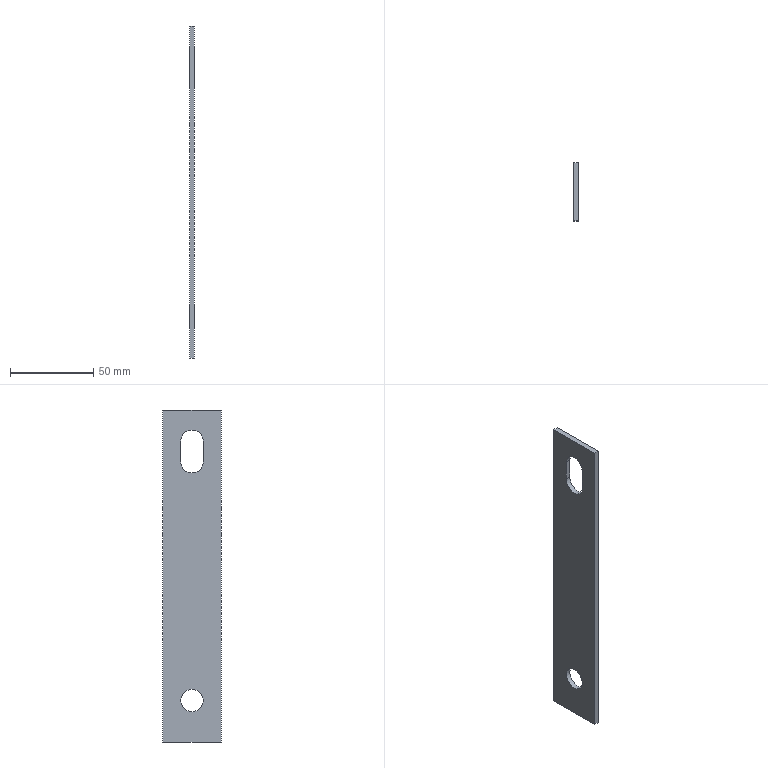Part | NX | features solid 2 | 1 solid | 11 faces | box 3 x 35 x 200 mm | volume 19635 mm3 | plane 8 | cylinder 3 | commonest cylinder face diameters 13.5 x3
STEP:
#1=CARTESIAN_POINT('',(1620.,-182.5,-320.));
#2=VERTEX_POINT('',#1);
#3=CARTESIAN_POINT('',(1620.,-182.5,-120.));
#4=VERTEX_POINT('',#3);
#5=CARTESIAN_POINT('',(1620.,-182.5,-320.));
#6=DIRECTION('',(0.,0.,1.));
#7=VECTOR('',#6,1000.);
#8=LINE('',#5,#7);
#9=EDGE_CURVE('',#2,#4,#8,.T.);
#10=ORIENTED_EDGE('',*,*,#9,.F.);
#11=CARTESIAN_POINT('',(1623.,-182.5,-320.));
#12=VERTEX_POINT('',#11);
#13=CARTESIAN_POINT('',(1623.,-182.5,-320.));
#14=DIRECTION('',(-1.,0.,0.));
#15=VECTOR('',#14,1000.);
#16=LINE('',#13,#15);
#17=EDGE_CURVE('',#12,#2,#16,.T.);
#18=ORIENTED_EDGE('',*,*,#17,.F.);
#19=CARTESIAN_POINT('',(1623.,-182.5,-120.));
#20=VERTEX_POINT('',#19);
#21=CARTESIAN_POINT('',(1623.,-182.5,-320.));
#22=DIRECTION('',(0.,0.,1.));
#23=VECTOR('',#22,1000.);
#24=LINE('',#21,#23);
#25=EDGE_CURVE('',#12,#20,#24,.T.);
#26=ORIENTED_EDGE('',*,*,#25,.T.);
#27=CARTESIAN_POINT('',(1623.,-182.5,-120.));
#28=DIRECTION('',(-1.,0.,0.));
#29=VECTOR('',#28,1000.);
#30=LINE('',#27,#29);
#31=EDGE_CURVE('',#20,#4,#30,.T.);
#32=ORIENTED_EDGE('',*,*,#31,.T.);
#33=EDGE_LOOP('',(#10,#18,#26,#32));
#34=FACE_BOUND('',#33,.T.);
#35=CARTESIAN_POINT('',(1623.,-182.5,-320.));
#36=DIRECTION('',(0.,-1.,0.));
#37=DIRECTION('',(0.,0.,1.));
#38=AXIS2_PLACEMENT_3D('',#35,#36,#37);
#39=PLANE('',#38);
#40=ADVANCED_FACE('',(#34),#39,.T.);
#41=CARTESIAN_POINT('',(1620.,-147.5,-120.));
#42=VERTEX_POINT('',#41);
#43=CARTESIAN_POINT('',(1620.,-182.5,-120.));
#44=DIRECTION('',(0.,1.,0.));
#45=VECTOR('',#44,1000.);
#46=LINE('',#43,#45);
#47=EDGE_CURVE('',#4,#42,#46,.T.);
#48=ORIENTED_EDGE('',*,*,#47,.F.);
#49=ORIENTED_EDGE('',*,*,#31,.F.);
#50=CARTESIAN_POINT('',(1623.,-147.5,-120.));
#51=VERTEX_POINT('',#50);
#52=CARTESIAN_POINT('',(1623.,-182.5,-120.));
#53=DIRECTION('',(0.,1.,0.));
#54=VECTOR('',#53,1000.);
#55=LINE('',#52,#54);
#56=EDGE_CURVE('',#20,#51,#55,.T.);
#57=ORIENTED_EDGE('',*,*,#56,.T.);
#58=CARTESIAN_POINT('',(1623.,-147.5,-120.));
#59=DIRECTION('',(-1.,0.,0.));
#60=VECTOR('',#59,1000.);
#61=LINE('',#58,#60);
#62=EDGE_CURVE('',#51,#42,#61,.T.);
#63=ORIENTED_EDGE('',*,*,#62,.T.);
#64=EDGE_LOOP('',(#48,#49,#57,#63));
#65=FACE_BOUND('',#64,.T.);
#66=CARTESIAN_POINT('',(1623.,-182.5,-120.));
#67=DIRECTION('',(0.,0.,1.));
#68=DIRECTION('',(-1.,0.,0.));
#69=AXIS2_PLACEMENT_3D('',#66,#67,#68);
#70=PLANE('',#69);
#71=ADVANCED_FACE('',(#65),#70,.T.);
#72=CARTESIAN_POINT('',(1620.,-147.5,-320.));
#73=VERTEX_POINT('',#72);
#74=CARTESIAN_POINT('',(1620.,-147.5,-120.));
#75=DIRECTION('',(0.,0.,-1.));
#76=VECTOR('',#75,1000.);
#77=LINE('',#74,#76);
#78=EDGE_CURVE('',#42,#73,#77,.T.);
#79=ORIENTED_EDGE('',*,*,#78,.F.);
#80=ORIENTED_EDGE('',*,*,#62,.F.);
#81=CARTESIAN_POINT('',(1623.,-147.5,-320.));
#82=VERTEX_POINT('',#81);
#83=CARTESIAN_POINT('',(1623.,-147.5,-120.));
#84=DIRECTION('',(0.,0.,-1.));
#85=VECTOR('',#84,1000.);
#86=LINE('',#83,#85);
#87=EDGE_CURVE('',#51,#82,#86,.T.);
#88=ORIENTED_EDGE('',*,*,#87,.T.);
#89=CARTESIAN_POINT('',(1623.,-147.5,-320.));
#90=DIRECTION('',(-1.,0.,0.));
#91=VECTOR('',#90,1000.);
#92=LINE('',#89,#91);
#93=EDGE_CURVE('',#82,#73,#92,.T.);
#94=ORIENTED_EDGE('',*,*,#93,.T.);
#95=EDGE_LOOP('',(#79,#80,#88,#94));
#96=FACE_BOUND('',#95,.T.);
#97=CARTESIAN_POINT('',(1623.,-147.5,-120.));
#98=DIRECTION('',(0.,1.,0.));
#99=DIRECTION('',(0.,0.,-1.));
#100=AXIS2_PLACEMENT_3D('',#97,#98,#99);
#101=PLANE('',#100);
#102=ADVANCED_FACE('',(#96),#101,.T.);
#103=CARTESIAN_POINT('',(1620.,-158.25,-151.25));
#104=VERTEX_POINT('',#103);
#105=CARTESIAN_POINT('',(1620.,-171.75,-151.25));
#106=VERTEX_POINT('',#105);
#107=CARTESIAN_POINT('',(1620.,-165.,-151.25));
#108=DIRECTION('',(-1.,0.,0.));
#109=DIRECTION('',(0.,-1.,0.));
#110=AXIS2_PLACEMENT_3D('',#107,#108,#109);
#111=CIRCLE('',#110,6.75);
#112=EDGE_CURVE('',#104,#106,#111,.T.);
#113=ORIENTED_EDGE('',*,*,#112,.T.);
#114=CARTESIAN_POINT('',(1623.,-171.75,-151.25));
#115=VERTEX_POINT('',#114);
#116=CARTESIAN_POINT('',(1623.,-171.75,-151.25));
#117=DIRECTION('',(-1.,0.,0.));
#118=VECTOR('',#117,1000.);
#119=LINE('',#116,#118);
#120=EDGE_CURVE('',#115,#106,#119,.T.);
#121=ORIENTED_EDGE('',*,*,#120,.F.);
#122=CARTESIAN_POINT('',(1623.,-158.25,-151.25));
#123=VERTEX_POINT('',#122);
#124=CARTESIAN_POINT('',(1623.,-165.,-151.25));
#125=DIRECTION('',(-1.,0.,0.));
#126=DIRECTION('',(0.,-1.,0.));
#127=AXIS2_PLACEMENT_3D('',#124,#125,#126);
#128=CIRCLE('',#127,6.75);
#129=EDGE_CURVE('',#123,#115,#128,.T.);
#130=ORIENTED_EDGE('',*,*,#129,.F.);
#131=CARTESIAN_POINT('',(1623.,-158.25,-151.25));
#132=DIRECTION('',(-1.,0.,0.));
#133=VECTOR('',#132,1000.);
#134=LINE('',#131,#133);
#135=EDGE_CURVE('',#123,#104,#134,.T.);
#136=ORIENTED_EDGE('',*,*,#135,.T.);
#137=EDGE_LOOP('',(#113,#121,#130,#136));
#138=FACE_BOUND('',#137,.T.);
#139=CARTESIAN_POINT('',(1623.,-165.,-151.25));
#140=DIRECTION('',(-1.,0.,0.));
#141=DIRECTION('',(0.,-1.,0.));
#142=AXIS2_PLACEMENT_3D('',#139,#140,#141);
#143=CYLINDRICAL_SURFACE('',#142,6.75);
#144=ADVANCED_FACE('',(#138),#143,.F.);
#145=CARTESIAN_POINT('',(1620.,-158.25,-138.75));
#146=VERTEX_POINT('',#145);
#147=CARTESIAN_POINT('',(1620.,-158.25,-151.25));
#148=DIRECTION('',(0.,0.,1.));
#149=VECTOR('',#148,1000.);
#150=LINE('',#147,#149);
#151=EDGE_CURVE('',#104,#146,#150,.T.);
#152=ORIENTED_EDGE('',*,*,#151,.F.);
#153=ORIENTED_EDGE('',*,*,#135,.F.);
#154=CARTESIAN_POINT('',(1623.,-158.25,-138.75));
#155=VERTEX_POINT('',#154);
#156=CARTESIAN_POINT('',(1623.,-158.25,-151.25));
#157=DIRECTION('',(0.,0.,1.));
#158=VECTOR('',#157,1000.);
#159=LINE('',#156,#158);
#160=EDGE_CURVE('',#123,#155,#159,.T.);
#161=ORIENTED_EDGE('',*,*,#160,.T.);
#162=CARTESIAN_POINT('',(1623.,-158.25,-138.75));
#163=DIRECTION('',(-1.,0.,0.));
#164=VECTOR('',#163,1000.);
#165=LINE('',#162,#164);
#166=EDGE_CURVE('',#155,#146,#165,.T.);
#167=ORIENTED_EDGE('',*,*,#166,.T.);
#168=EDGE_LOOP('',(#152,#153,#161,#167));
#169=FACE_BOUND('',#168,.T.);
#170=CARTESIAN_POINT('',(1623.,-158.25,-151.25));
#171=DIRECTION('',(0.,-1.,0.));
#172=DIRECTION('',(1.,0.,0.));
#173=AXIS2_PLACEMENT_3D('',#170,#171,#172);
#174=PLANE('',#173);
#175=ADVANCED_FACE('',(#169),#174,.T.);
#176=CARTESIAN_POINT('',(1620.,-171.75,-138.75));
#177=VERTEX_POINT('',#176);
#178=CARTESIAN_POINT('',(1620.,-165.,-138.75));
#179=DIRECTION('',(-1.,0.,0.));
#180=DIRECTION('',(0.,-1.,0.));
#181=AXIS2_PLACEMENT_3D('',#178,#179,#180);
#182=CIRCLE('',#181,6.75);
#183=EDGE_CURVE('',#177,#146,#182,.T.);
#184=ORIENTED_EDGE('',*,*,#183,.T.);
#185=ORIENTED_EDGE('',*,*,#166,.F.);
#186=CARTESIAN_POINT('',(1623.,-171.75,-138.75));
#187=VERTEX_POINT('',#186);
#188=CARTESIAN_POINT('',(1623.,-165.,-138.75));
#189=DIRECTION('',(-1.,0.,0.));
#190=DIRECTION('',(0.,-1.,0.));
#191=AXIS2_PLACEMENT_3D('',#188,#189,#190);
#192=CIRCLE('',#191,6.75);
#193=EDGE_CURVE('',#187,#155,#192,.T.);
#194=ORIENTED_EDGE('',*,*,#193,.F.);
#195=CARTESIAN_POINT('',(1623.,-171.75,-138.75));
#196=DIRECTION('',(-1.,0.,0.));
#197=VECTOR('',#196,1000.);
#198=LINE('',#195,#197);
#199=EDGE_CURVE('',#187,#177,#198,.T.);
#200=ORIENTED_EDGE('',*,*,#199,.T.);
#201=EDGE_LOOP('',(#184,#185,#194,#200));
#202=FACE_BOUND('',#201,.T.);
#203=CARTESIAN_POINT('',(1623.,-165.,-138.75));
#204=DIRECTION('',(-1.,0.,0.));
#205=DIRECTION('',(0.,-1.,0.));
#206=AXIS2_PLACEMENT_3D('',#203,#204,#205);
#207=CYLINDRICAL_SURFACE('',#206,6.75);
#208=ADVANCED_FACE('',(#202),#207,.F.);
#209=CARTESIAN_POINT('',(1620.,-171.75,-138.75));
#210=DIRECTION('',(0.,0.,-1.));
#211=VECTOR('',#210,1000.);
#212=LINE('',#209,#211);
#213=EDGE_CURVE('',#177,#106,#212,.T.);
#214=ORIENTED_EDGE('',*,*,#213,.F.);
#215=ORIENTED_EDGE('',*,*,#199,.F.);
#216=CARTESIAN_POINT('',(1623.,-171.75,-138.75));
#217=DIRECTION('',(0.,0.,-1.));
#218=VECTOR('',#217,1000.);
#219=LINE('',#216,#218);
#220=EDGE_CURVE('',#187,#115,#219,.T.);
#221=ORIENTED_EDGE('',*,*,#220,.T.);
#222=ORIENTED_EDGE('',*,*,#120,.T.);
#223=EDGE_LOOP('',(#214,#215,#221,#222));
#224=FACE_BOUND('',#223,.T.);
#225=CARTESIAN_POINT('',(1623.,-171.75,-138.75));
#226=DIRECTION('',(0.,1.,0.));
#227=DIRECTION('',(-1.,0.,0.));
#228=AXIS2_PLACEMENT_3D('',#225,#226,#227);
#229=PLANE('',#228);
#230=ADVANCED_FACE('',(#224),#229,.T.);
#231=CARTESIAN_POINT('',(1623.,-171.75,-295.));
#232=VERTEX_POINT('',#231);
#233=CARTESIAN_POINT('',(1623.,-165.,-295.));
#234=DIRECTION('',(-1.,0.,0.));
#235=DIRECTION('',(0.,-1.,0.));
#236=AXIS2_PLACEMENT_3D('',#233,#234,#235);
#237=CIRCLE('',#236,6.75);
#238=EDGE_CURVE('',#232,#232,#237,.T.);
#239=ORIENTED_EDGE('',*,*,#238,.F.);
#240=EDGE_LOOP('',(#239));
#241=FACE_BOUND('',#240,.T.);
#242=CARTESIAN_POINT('',(1620.,-171.75,-295.));
#243=VERTEX_POINT('',#242);
#244=CARTESIAN_POINT('',(1620.,-165.,-295.));
#245=DIRECTION('',(-1.,0.,0.));
#246=DIRECTION('',(0.,-1.,0.));
#247=AXIS2_PLACEMENT_3D('',#244,#245,#246);
#248=CIRCLE('',#247,6.75);
#249=EDGE_CURVE('',#243,#243,#248,.T.);
#250=ORIENTED_EDGE('',*,*,#249,.T.);
#251=EDGE_LOOP('',(#250));
#252=FACE_BOUND('',#251,.T.);
#253=CARTESIAN_POINT('',(1623.,-165.,-295.));
#254=DIRECTION('',(-1.,0.,0.));
#255=DIRECTION('',(0.,-1.,0.));
#256=AXIS2_PLACEMENT_3D('',#253,#254,#255);
#257=CYLINDRICAL_SURFACE('',#256,6.75);
#258=ADVANCED_FACE('',(#241,#252),#257,.F.);
#259=CARTESIAN_POINT('',(1620.,-147.5,-320.));
#260=DIRECTION('',(0.,-1.,0.));
#261=VECTOR('',#260,1000.);
#262=LINE('',#259,#261);
#263=EDGE_CURVE('',#73,#2,#262,.T.);
#264=ORIENTED_EDGE('',*,*,#263,.F.);
#265=ORIENTED_EDGE('',*,*,#93,.F.);
#266=CARTESIAN_POINT('',(1623.,-147.5,-320.));
#267=DIRECTION('',(0.,-1.,0.));
#268=VECTOR('',#267,1000.);
#269=LINE('',#266,#268);
#270=EDGE_CURVE('',#82,#12,#269,.T.);
#271=ORIENTED_EDGE('',*,*,#270,.T.);
#272=ORIENTED_EDGE('',*,*,#17,.T.);
#273=EDGE_LOOP('',(#264,#265,#271,#272));
#274=FACE_BOUND('',#273,.T.);
#275=CARTESIAN_POINT('',(1623.,-147.5,-320.));
#276=DIRECTION('',(0.,0.,-1.));
#277=DIRECTION('',(1.,0.,0.));
#278=AXIS2_PLACEMENT_3D('',#275,#276,#277);
#279=PLANE('',#278);
#280=ADVANCED_FACE('',(#274),#279,.T.);
#281=ORIENTED_EDGE('',*,*,#238,.T.);
#282=EDGE_LOOP('',(#281));
#283=FACE_BOUND('',#282,.T.);
#284=ORIENTED_EDGE('',*,*,#129,.T.);
#285=ORIENTED_EDGE('',*,*,#220,.F.);
#286=ORIENTED_EDGE('',*,*,#193,.T.);
#287=ORIENTED_EDGE('',*,*,#160,.F.);
#288=EDGE_LOOP('',(#284,#285,#286,#287));
#289=FACE_BOUND('',#288,.T.);
#290=ORIENTED_EDGE('',*,*,#25,.F.);
#291=ORIENTED_EDGE('',*,*,#270,.F.);
#292=ORIENTED_EDGE('',*,*,#87,.F.);
#293=ORIENTED_EDGE('',*,*,#56,.F.);
#294=EDGE_LOOP('',(#290,#291,#292,#293));
#295=FACE_BOUND('',#294,.T.);
#296=CARTESIAN_POINT('',(1623.,-182.5,-120.));
#297=DIRECTION('',(-1.,0.,0.));
#298=DIRECTION('',(0.,-1.,0.));
#299=AXIS2_PLACEMENT_3D('',#296,#297,#298);
#300=PLANE('',#299);
#301=ADVANCED_FACE('',(#283,#289,#295),#300,.F.);
#302=ORIENTED_EDGE('',*,*,#249,.F.);
#303=EDGE_LOOP('',(#302));
#304=FACE_BOUND('',#303,.T.);
#305=ORIENTED_EDGE('',*,*,#112,.F.);
#306=ORIENTED_EDGE('',*,*,#151,.T.);
#307=ORIENTED_EDGE('',*,*,#183,.F.);
#308=ORIENTED_EDGE('',*,*,#213,.T.);
#309=EDGE_LOOP('',(#305,#306,#307,#308));
#310=FACE_BOUND('',#309,.T.);
#311=ORIENTED_EDGE('',*,*,#9,.T.);
#312=ORIENTED_EDGE('',*,*,#47,.T.);
#313=ORIENTED_EDGE('',*,*,#78,.T.);
#314=ORIENTED_EDGE('',*,*,#263,.T.);
#315=EDGE_LOOP('',(#311,#312,#313,#314));
#316=FACE_BOUND('',#315,.T.);
#317=CARTESIAN_POINT('',(1620.,-182.5,-120.));
#318=DIRECTION('',(-1.,0.,0.));
#319=DIRECTION('',(0.,-1.,0.));
#320=AXIS2_PLACEMENT_3D('',#317,#318,#319);
#321=PLANE('',#320);
#322=ADVANCED_FACE('',(#304,#310,#316),#321,.T.);
#323=CLOSED_SHELL('',(#40,#71,#102,#144,#175,#208,#230,#258,#280,#301,#322));
#324=MANIFOLD_SOLID_BREP('',#323);
#325=(LENGTH_UNIT()NAMED_UNIT(*)SI_UNIT(.MILLI.,.METRE.));
#326=UNCERTAINTY_MEASURE_WITH_UNIT(LENGTH_MEASURE(0.00001),#325,'','');
#327=(NAMED_UNIT(*)PLANE_ANGLE_UNIT()SI_UNIT($,.RADIAN.));
#328=(NAMED_UNIT(*)SI_UNIT($,.STERADIAN.)SOLID_ANGLE_UNIT());
#329=(GEOMETRIC_REPRESENTATION_CONTEXT(3)GLOBAL_UNCERTAINTY_ASSIGNED_CONTEXT((#326))GLOBAL_UNIT_ASSIGNED_CONTEXT((#325,#327,#328))REPRESENTATION_CONTEXT('',''));
#330=ADVANCED_BREP_SHAPE_REPRESENTATION('',(#324),#329);